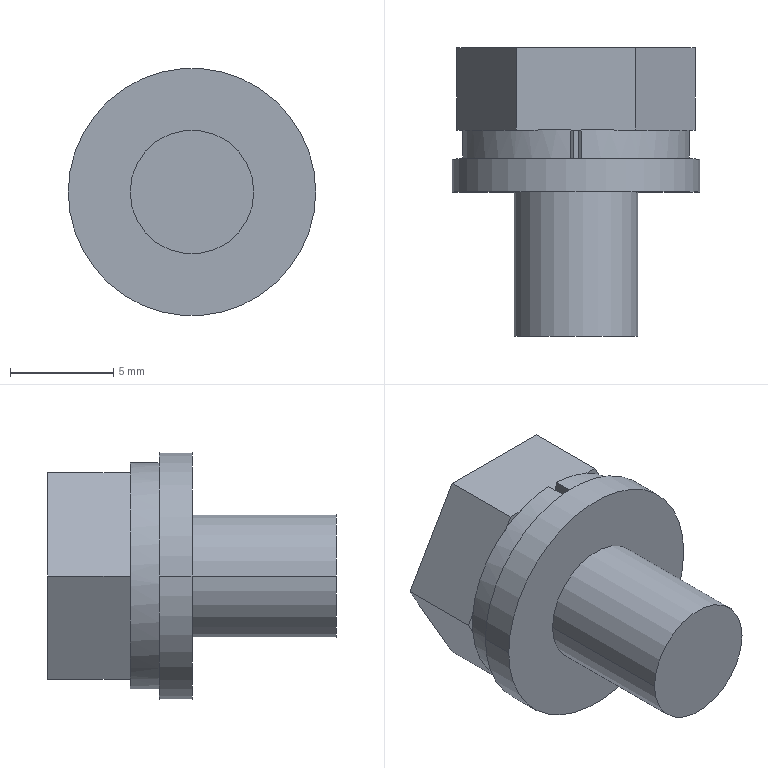Part | STEP file | LIB_36623098_M6X10 | 1 solid | 45 faces | box 12 x 14 x 12 mm | volume 823.04 mm3 | plane 27 | cylinder 18 | commonest cylinder face diameters 0.809 x6 2 x6 6 x3 12 x2 11 x1